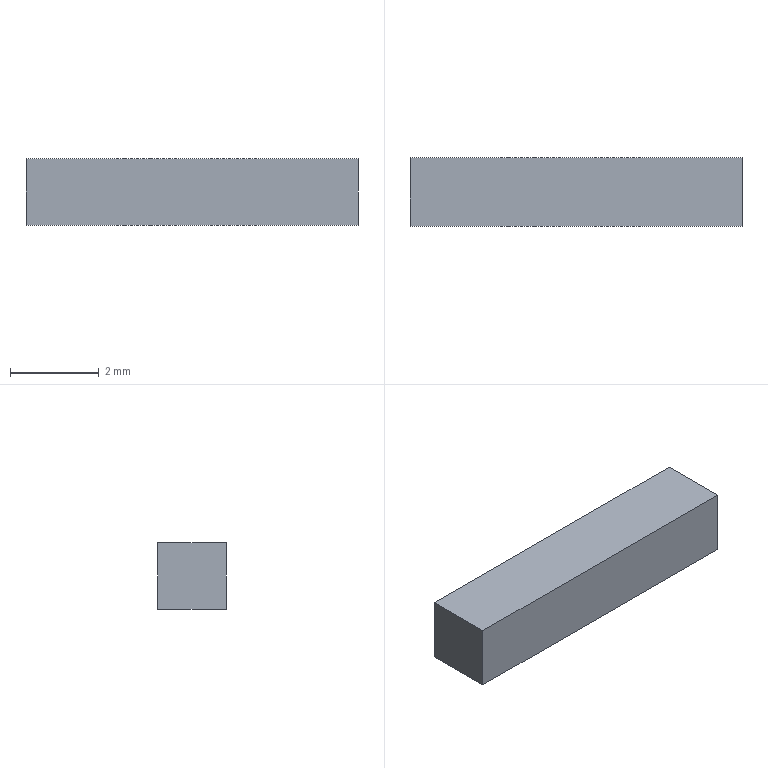Part | Creo | 1 solid | 6 faces | box 7.5 x 1.55 x 1.5 mm | volume 17.437 mm3 | plane 6
STEP:
#1=CARTESIAN_POINT('',(0.,0.,0.));
#2=DIRECTION('',(0.,0.,1.));
#3=DIRECTION('',(1.,0.,0.));
#4=AXIS2_PLACEMENT_3D('',#1,#2,#3);
#5=CARTESIAN_POINT('',(-3.75,-0.775,0.));
#6=VERTEX_POINT('',#5);
#7=CARTESIAN_POINT('',(3.75,-0.775,0.));
#8=VERTEX_POINT('',#7);
#9=CARTESIAN_POINT('',(-3.75,-0.775,0.));
#10=DIRECTION('',(1.,0.,0.));
#11=VECTOR('',#10,7.5);
#12=LINE('',#9,#11);
#13=EDGE_CURVE('',#6,#8,#12,.T.);
#14=ORIENTED_EDGE('',*,*,#13,.T.);
#15=CARTESIAN_POINT('',(3.75,0.775,0.));
#16=VERTEX_POINT('',#15);
#17=CARTESIAN_POINT('',(3.75,-0.775,0.));
#18=DIRECTION('',(0.,1.,0.));
#19=VECTOR('',#18,1.55);
#20=LINE('',#17,#19);
#21=EDGE_CURVE('',#8,#16,#20,.T.);
#22=ORIENTED_EDGE('',*,*,#21,.T.);
#23=CARTESIAN_POINT('',(-3.75,0.775,0.));
#24=VERTEX_POINT('',#23);
#25=CARTESIAN_POINT('',(3.75,0.775,0.));
#26=DIRECTION('',(-1.,0.,0.));
#27=VECTOR('',#26,7.5);
#28=LINE('',#25,#27);
#29=EDGE_CURVE('',#16,#24,#28,.T.);
#30=ORIENTED_EDGE('',*,*,#29,.T.);
#31=CARTESIAN_POINT('',(-3.75,0.775,0.));
#32=DIRECTION('',(0.,-1.,0.));
#33=VECTOR('',#32,1.55);
#34=LINE('',#31,#33);
#35=EDGE_CURVE('',#24,#6,#34,.T.);
#36=ORIENTED_EDGE('',*,*,#35,.T.);
#37=EDGE_LOOP('',(#14,#22,#30,#36));
#38=FACE_OUTER_BOUND('',#37,.F.);
#39=CARTESIAN_POINT('',(0.,0.,0.));
#40=DIRECTION('',(0.,0.,1.));
#41=DIRECTION('',(1.,0.,0.));
#42=AXIS2_PLACEMENT_3D('',#39,#40,#41);
#43=PLANE('',#42);
#44=ADVANCED_FACE('',(#38),#43,.F.);
#45=ORIENTED_EDGE('',*,*,#13,.F.);
#46=CARTESIAN_POINT('',(-3.75,-0.775,1.5));
#47=VERTEX_POINT('',#46);
#48=CARTESIAN_POINT('',(-3.75,-0.775,0.));
#49=DIRECTION('',(0.,0.,1.));
#50=VECTOR('',#49,1.5);
#51=LINE('',#48,#50);
#52=EDGE_CURVE('',#6,#47,#51,.T.);
#53=ORIENTED_EDGE('',*,*,#52,.T.);
#54=CARTESIAN_POINT('',(3.75,-0.775,1.5));
#55=VERTEX_POINT('',#54);
#56=CARTESIAN_POINT('',(-3.75,-0.775,1.5));
#57=DIRECTION('',(1.,0.,0.));
#58=VECTOR('',#57,7.5);
#59=LINE('',#56,#58);
#60=EDGE_CURVE('',#47,#55,#59,.T.);
#61=ORIENTED_EDGE('',*,*,#60,.T.);
#62=CARTESIAN_POINT('',(3.75,-0.775,0.));
#63=DIRECTION('',(0.,0.,1.));
#64=VECTOR('',#63,1.5);
#65=LINE('',#62,#64);
#66=EDGE_CURVE('',#8,#55,#65,.T.);
#67=ORIENTED_EDGE('',*,*,#66,.F.);
#68=EDGE_LOOP('',(#45,#53,#61,#67));
#69=FACE_OUTER_BOUND('',#68,.F.);
#70=CARTESIAN_POINT('',(-3.75,-0.775,0.));
#71=DIRECTION('',(0.,-1.,0.));
#72=DIRECTION('',(1.,0.,0.));
#73=AXIS2_PLACEMENT_3D('',#70,#71,#72);
#74=PLANE('',#73);
#75=ADVANCED_FACE('',(#69),#74,.T.);
#76=ORIENTED_EDGE('',*,*,#35,.F.);
#77=CARTESIAN_POINT('',(-3.75,0.775,1.5));
#78=VERTEX_POINT('',#77);
#79=CARTESIAN_POINT('',(-3.75,0.775,0.));
#80=DIRECTION('',(0.,0.,1.));
#81=VECTOR('',#80,1.5);
#82=LINE('',#79,#81);
#83=EDGE_CURVE('',#24,#78,#82,.T.);
#84=ORIENTED_EDGE('',*,*,#83,.T.);
#85=CARTESIAN_POINT('',(-3.75,0.775,1.5));
#86=DIRECTION('',(0.,-1.,0.));
#87=VECTOR('',#86,1.55);
#88=LINE('',#85,#87);
#89=EDGE_CURVE('',#78,#47,#88,.T.);
#90=ORIENTED_EDGE('',*,*,#89,.T.);
#91=ORIENTED_EDGE('',*,*,#52,.F.);
#92=EDGE_LOOP('',(#76,#84,#90,#91));
#93=FACE_OUTER_BOUND('',#92,.F.);
#94=CARTESIAN_POINT('',(-3.75,0.775,0.));
#95=DIRECTION('',(-1.,0.,0.));
#96=DIRECTION('',(0.,-1.,0.));
#97=AXIS2_PLACEMENT_3D('',#94,#95,#96);
#98=PLANE('',#97);
#99=ADVANCED_FACE('',(#93),#98,.T.);
#100=ORIENTED_EDGE('',*,*,#29,.F.);
#101=CARTESIAN_POINT('',(3.75,0.775,1.5));
#102=VERTEX_POINT('',#101);
#103=CARTESIAN_POINT('',(3.75,0.775,0.));
#104=DIRECTION('',(0.,0.,1.));
#105=VECTOR('',#104,1.5);
#106=LINE('',#103,#105);
#107=EDGE_CURVE('',#16,#102,#106,.T.);
#108=ORIENTED_EDGE('',*,*,#107,.T.);
#109=CARTESIAN_POINT('',(3.75,0.775,1.5));
#110=DIRECTION('',(-1.,0.,0.));
#111=VECTOR('',#110,7.5);
#112=LINE('',#109,#111);
#113=EDGE_CURVE('',#102,#78,#112,.T.);
#114=ORIENTED_EDGE('',*,*,#113,.T.);
#115=ORIENTED_EDGE('',*,*,#83,.F.);
#116=EDGE_LOOP('',(#100,#108,#114,#115));
#117=FACE_OUTER_BOUND('',#116,.F.);
#118=CARTESIAN_POINT('',(3.75,0.775,0.));
#119=DIRECTION('',(0.,1.,0.));
#120=DIRECTION('',(-1.,0.,0.));
#121=AXIS2_PLACEMENT_3D('',#118,#119,#120);
#122=PLANE('',#121);
#123=ADVANCED_FACE('',(#117),#122,.T.);
#124=ORIENTED_EDGE('',*,*,#21,.F.);
#125=ORIENTED_EDGE('',*,*,#66,.T.);
#126=CARTESIAN_POINT('',(3.75,-0.775,1.5));
#127=DIRECTION('',(0.,1.,0.));
#128=VECTOR('',#127,1.55);
#129=LINE('',#126,#128);
#130=EDGE_CURVE('',#55,#102,#129,.T.);
#131=ORIENTED_EDGE('',*,*,#130,.T.);
#132=ORIENTED_EDGE('',*,*,#107,.F.);
#133=EDGE_LOOP('',(#124,#125,#131,#132));
#134=FACE_OUTER_BOUND('',#133,.F.);
#135=CARTESIAN_POINT('',(3.75,-0.775,0.));
#136=DIRECTION('',(1.,0.,0.));
#137=DIRECTION('',(0.,1.,0.));
#138=AXIS2_PLACEMENT_3D('',#135,#136,#137);
#139=PLANE('',#138);
#140=ADVANCED_FACE('',(#134),#139,.T.);
#141=ORIENTED_EDGE('',*,*,#60,.F.);
#142=ORIENTED_EDGE('',*,*,#89,.F.);
#143=ORIENTED_EDGE('',*,*,#113,.F.);
#144=ORIENTED_EDGE('',*,*,#130,.F.);
#145=EDGE_LOOP('',(#141,#142,#143,#144));
#146=FACE_OUTER_BOUND('',#145,.F.);
#147=CARTESIAN_POINT('',(0.,0.,1.5));
#148=DIRECTION('',(0.,0.,1.));
#149=DIRECTION('',(1.,0.,0.));
#150=AXIS2_PLACEMENT_3D('',#147,#148,#149);
#151=PLANE('',#150);
#152=ADVANCED_FACE('',(#146),#151,.T.);
#153=CLOSED_SHELL('',(#44,#75,#99,#123,#140,#152));
#154=MANIFOLD_SOLID_BREP('',#153);
#155=(LENGTH_UNIT()NAMED_UNIT(*)SI_UNIT(.MILLI.,.METRE.));
#156=UNCERTAINTY_MEASURE_WITH_UNIT(LENGTH_MEASURE(0.0007804),#155,'','');
#157=(NAMED_UNIT(*)PLANE_ANGLE_UNIT()SI_UNIT($,.RADIAN.));
#158=PLANE_ANGLE_MEASURE_WITH_UNIT(PLANE_ANGLE_MEASURE(0.01745),#157);
#159=(CONVERSION_BASED_UNIT('DEGREE',#158)NAMED_UNIT(*)PLANE_ANGLE_UNIT());
#160=(NAMED_UNIT(*)SI_UNIT($,.STERADIAN.)SOLID_ANGLE_UNIT());
#161=(GEOMETRIC_REPRESENTATION_CONTEXT(3)GLOBAL_UNCERTAINTY_ASSIGNED_CONTEXT((#156))GLOBAL_UNIT_ASSIGNED_CONTEXT((#155,#159,#160))REPRESENTATION_CONTEXT('',''));
#162=ADVANCED_BREP_SHAPE_REPRESENTATION('',(#4,#154),#161);